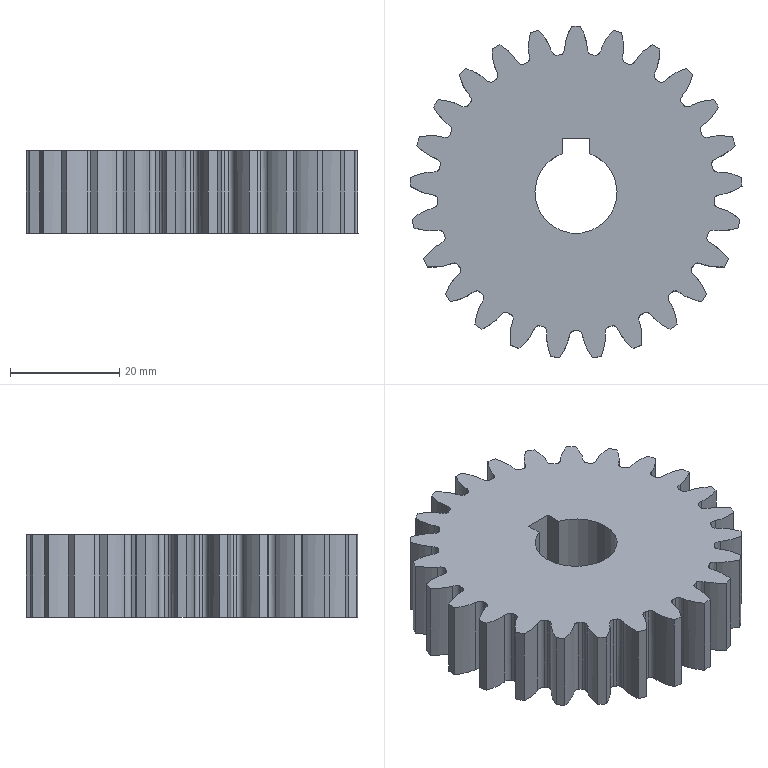Part | SolidWorks | features BaseBody 1, ICE 1 | 1 solid | 156 faces | box 60.71 x 60.601 x 15 mm | volume 33960 mm3 | spline 125 | cylinder 26 | plane 5 | commonest cylinder face diameters 50.625 x25 15 x1